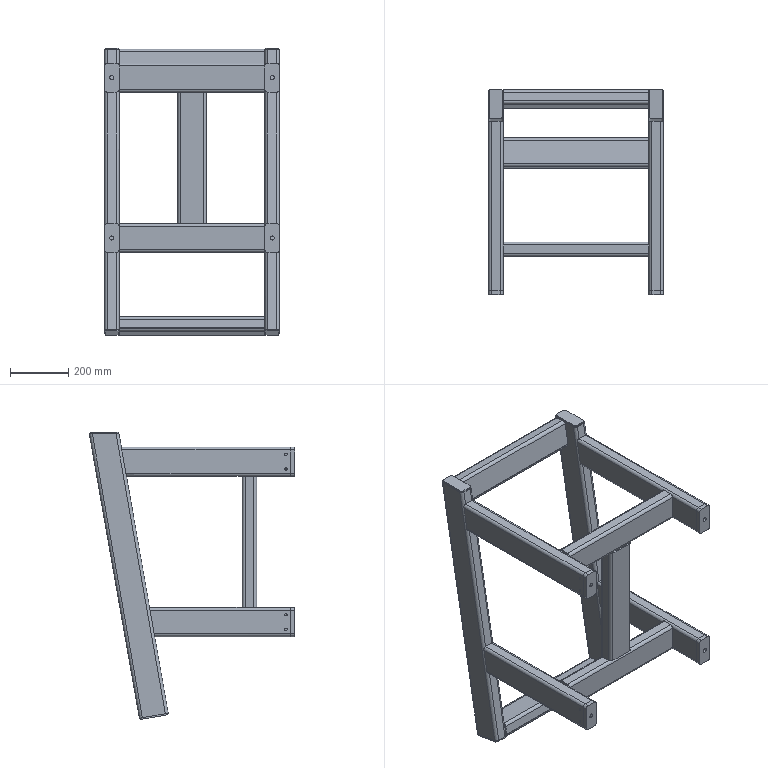Part | STEP file | PN_0032_storage rack_default_machined_ | 19 solids | 322 faces | box 600 x 704.072 x 984.374 mm | volume 9049621 mm3 | plane 174 | cylinder 148 | commonest cylinder face diameters 20 x62 10 x46 8.5 x32 14 x8